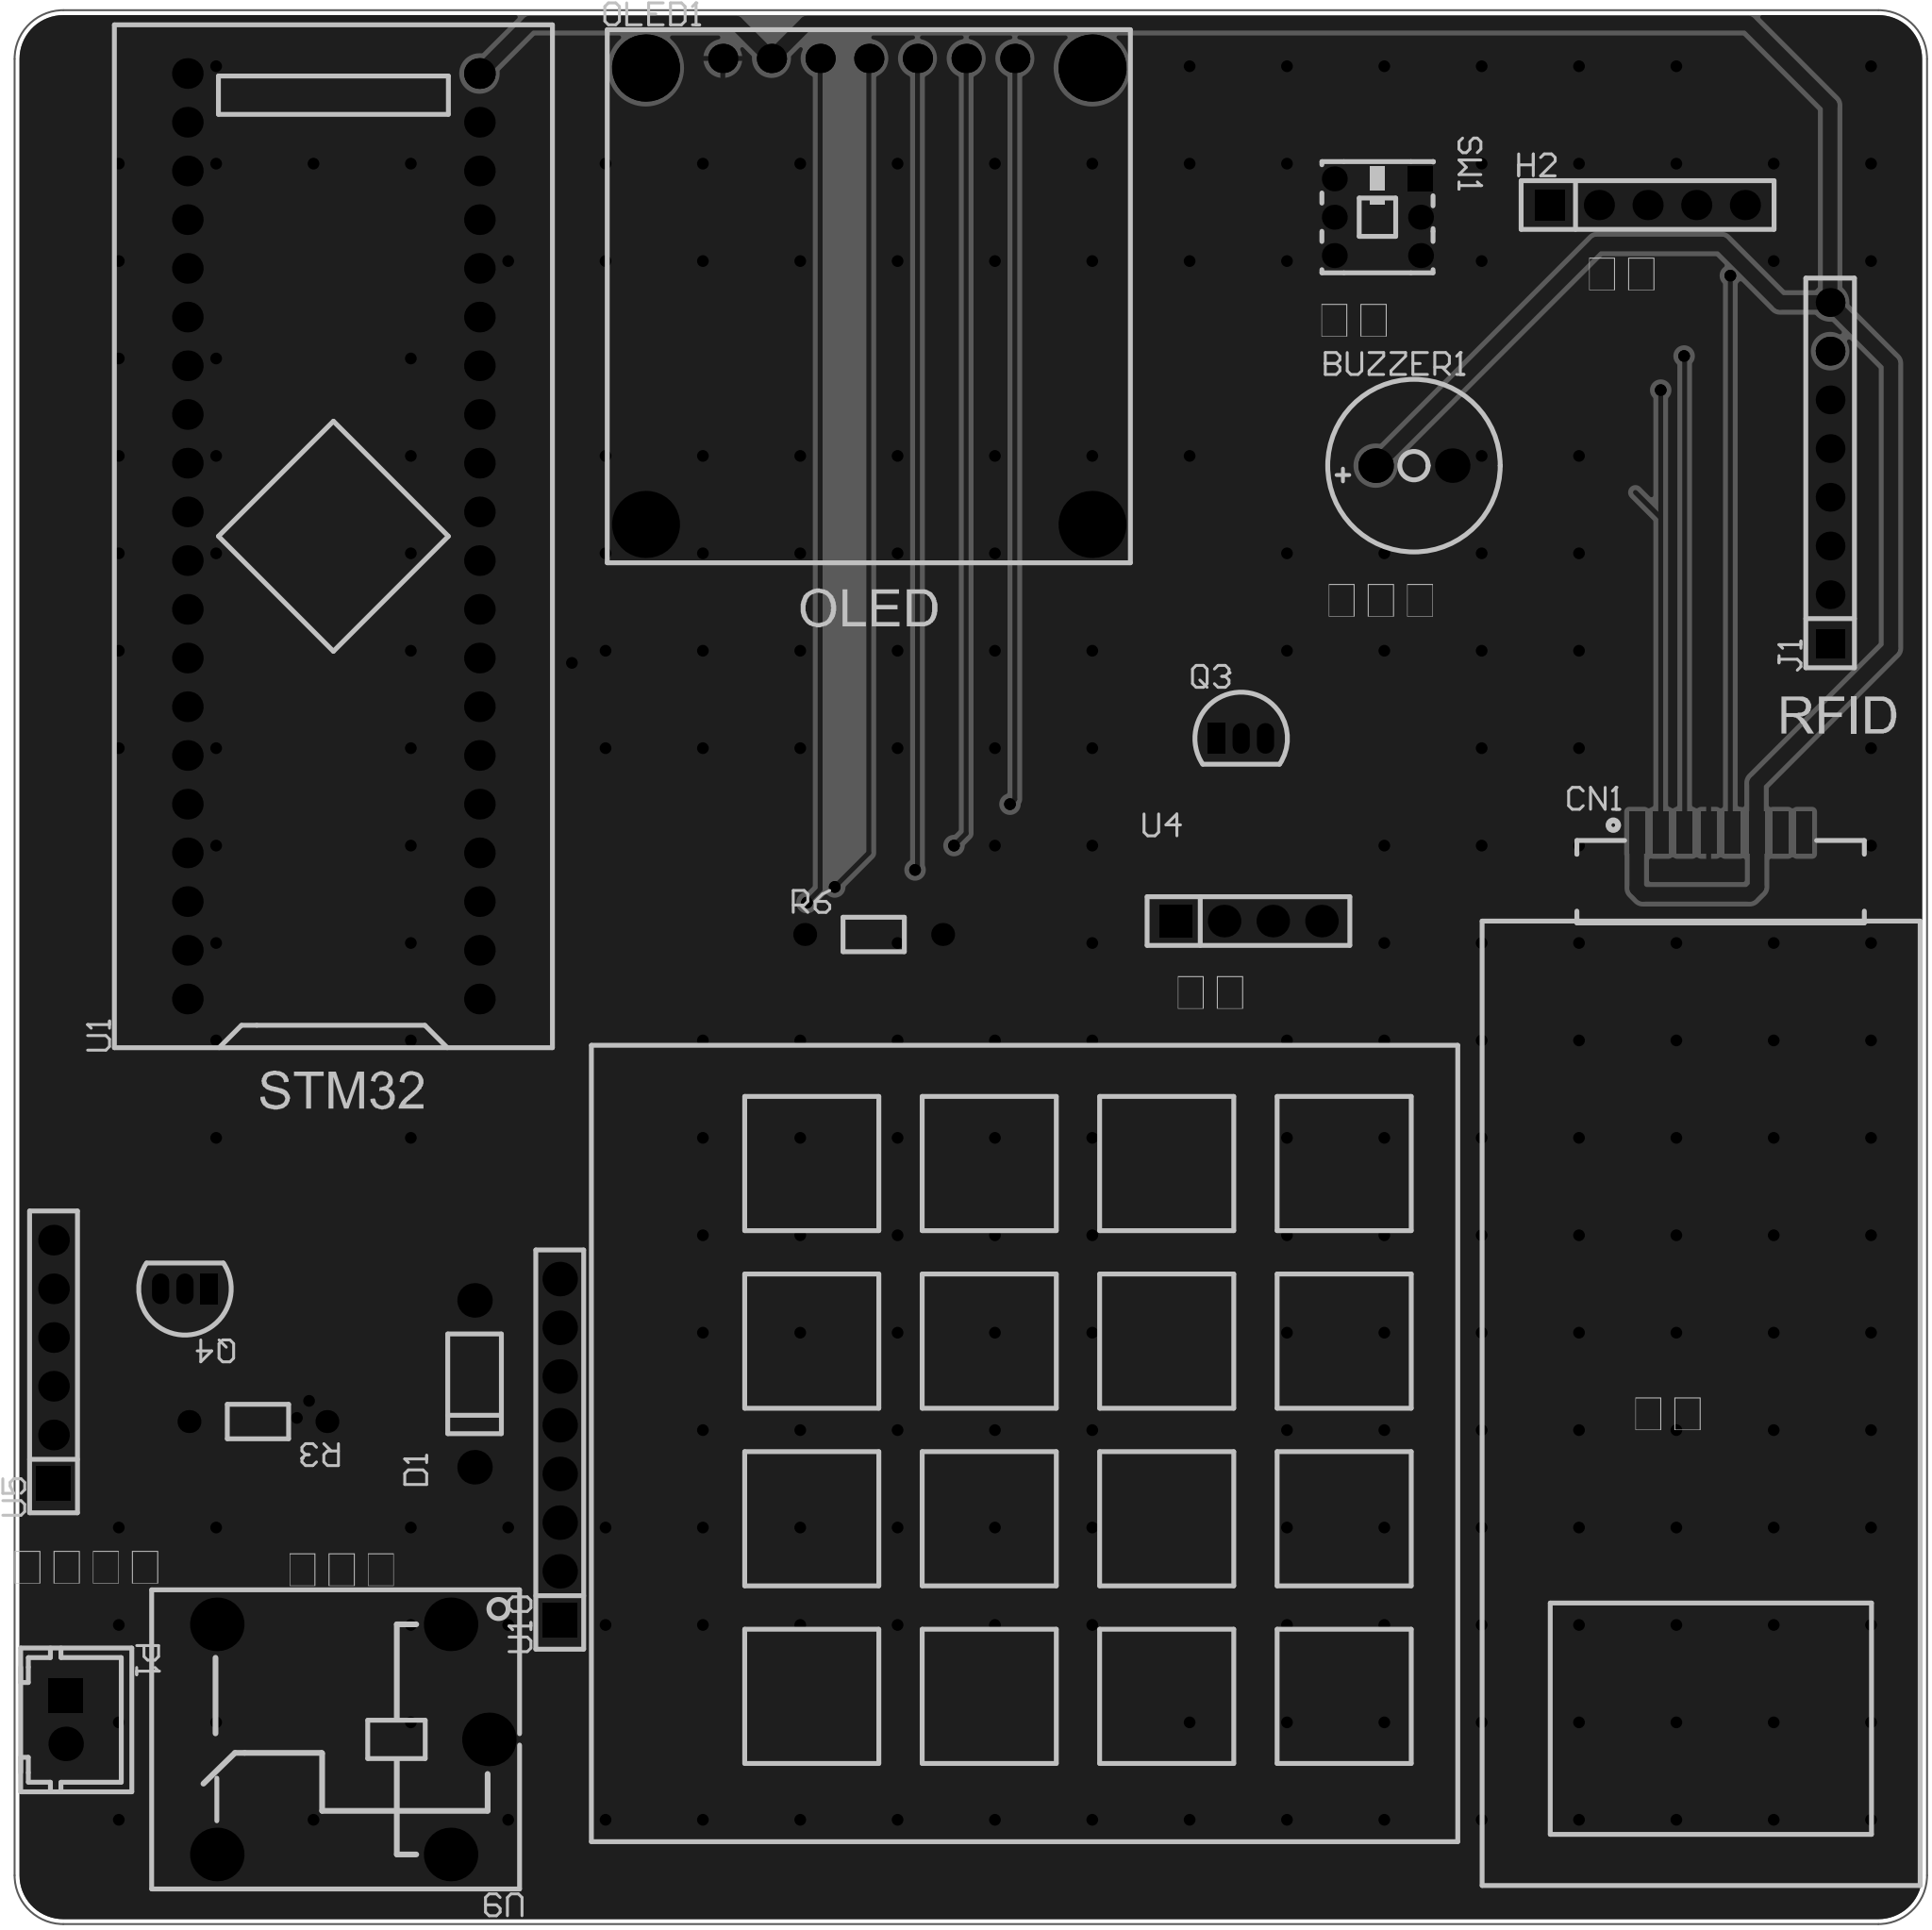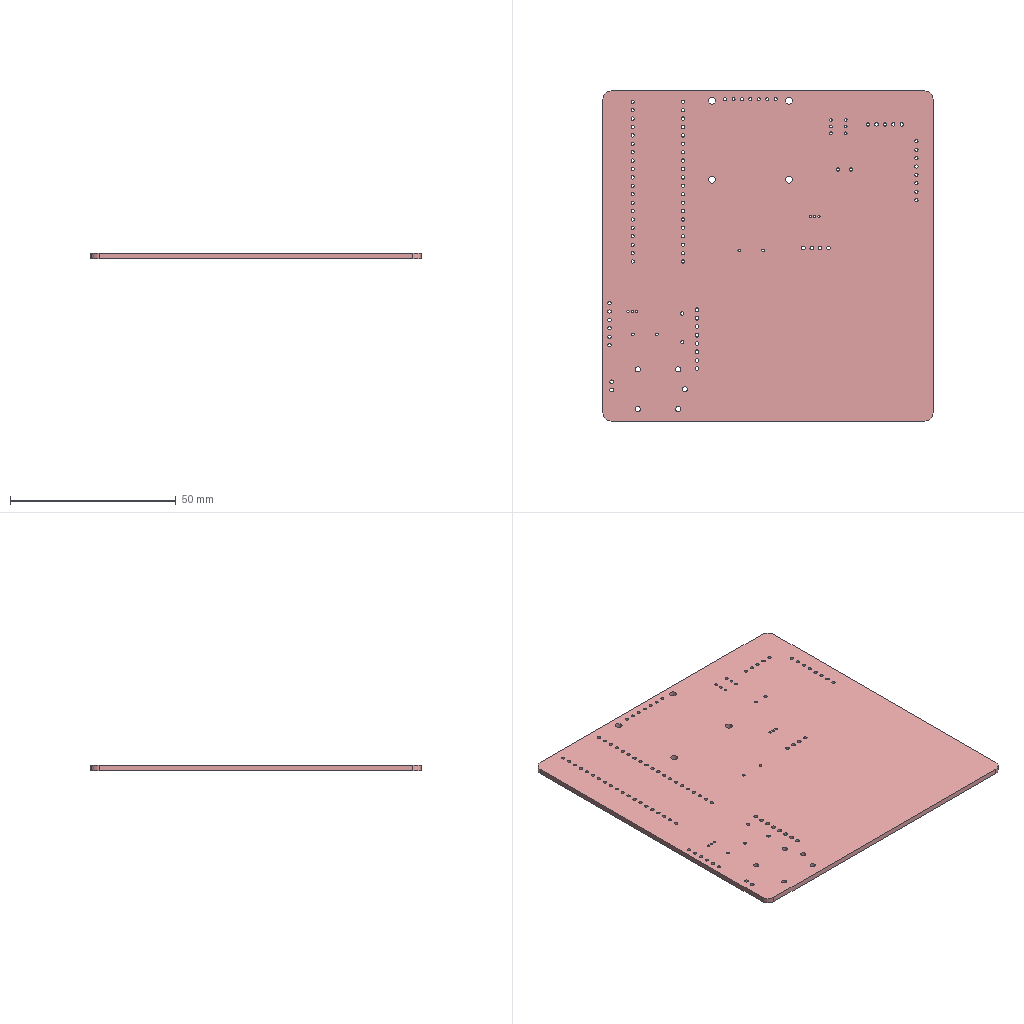Circuit board layout | Altium Designer | box 99.8 x 99.8 x 1.6 mm
Layer stack:
# Altium Designer layer stack of  (unit mm; dielectric type: 0 none, 1 core, 2 prepreg, 3 surface material)
index,name,kind,layer,copper_thickness_mm,dielectric_type,dielectric_thickness_mm,dielectric_material,dielectric_constant
0,Top Paste Mask Layer,other,,,,,,
1,Top Silkscreen Layer,other,,,,,,
2,Top Solder Mask Layer,dielectric,,,3,0.01,,3.3
3,Top Layer,copper,Top Layer,0.035,,,,
4,Dielectric1,dielectric,,,3,1.51,FR4,4.5
5,Bottom Layer,copper,Bottom Layer,0.035,,,,
6,Bottom Solder Mask Layer,dielectric,,,3,0.01,,3.3
7,Bottom Silkscreen Layer,other,,,,,,
8,Bottom Paste Mask Layer,other,,,,,,
# drill layer pairs: low layer,high layer
drill_pair,Top Layer,Bottom Layer
Part placement:
Designator,Comment,Layer,Footprint,Center-X(mm),Center-Y(mm),Rotation
J1,,TopLayer,HDR-TH_8P-P2.54-V-M,175.387,153.924,90
OLED1,,TopLayer,0.96OLED,125.222,163.388,0
U10,,TopLayer,HDR-TH_8P-P2.54-V-F-1,109.093,102.997,90
U1,LCKFB-DKX-STM32F103C8T6,TopLayer,CONN-TH_L53.3-W22.9_STM32F103C8T6-CARD,97.282,150.622,90
U4,,TopLayer,HDR-TH_4P-P2.54-V-F,145.034,130.556,0
Q4,,TopLayer,S8050_TO_92,89.535,111.379,180
R3,1K,TopLayer,Res_1/8W,93.345,104.458,180
D1,,TopLayer,DO_1N4007,104.648,106.426,90
U9,SRD-12VDC-SL-C,TopLayer,RELAY-TH_SRD-XXVDC-XL-C,98.298,87.884,180
R6,1K,TopLayer,Res_1/8W,125.476,129.857,0
BUZZER1,2.7kHz,TopLayer,BUZ-TH_BD9.0-P4.00-D0.6-FD,153.67,154.305,0
Q3,,TopLayer,S8050_TO_92,144.653,140.081,0
H2,,TopLayer,HDR-TH_5P-P2.54-V-F,165.862,167.894,0
P1,WAFER-XH254Z-2A,TopLayer,CONN-TH_2P-P2.50_XH-2A_3045048,83.312,88.9,270
SW1,5.8 WSPT,TopLayer,SW-TH_6P-L5.8-W5.8-P2.00-LS4.5-TL_K8-5851E-L1,151.765,167.259,270
U5,,TopLayer,HDR-TH_6P-P2.54-V-F,82.677,107.569,90
CN1,AS608,TopLayer,AS608,169.672,133.858,0
Pad and via stacks:
# Altium Designer via and pad stacks of  (unit mm). Each distinct definition once, with the count of objects using it.
# via: kind,start_layer,end_layer,hole_mm,diameter_mm,mode(0 simple;1 top-mid-bottom;2 full stack),diameter_per_layer,count,example_net
# pad: kind,layer,hole_mm,hole_type(0 round;1 square;2 slot),plating,top_size,top_shape(1 round;2 rect;3 octagon;9 rounded rect),mid_size,bottom_size,mode,footprint,size_per_layer,count,example
pad,Multi-Layer,1,0,plated,1.5x1.5,2,1.5x1.5,1.5x1.5,0,HDR-TH_8P-P2.54-V-M,,1,J1.1
pad,Multi-Layer,1,0,plated,1.5x1.5,1,1.5x1.5,1.5x1.5,0,HDR-TH_8P-P2.54-V-M,,7,J1.2
pad,Multi-Layer,0.9144,0,plated,1.524x1.524,1,1.524x1.524,1.524x1.524,0,0.96OLED,,7,OLED1.1
pad,Multi-Layer,2.1,0,plated,3.5x3.5,1,3.5x3.5,3.5x3.5,0,0.96OLED,,4,OLED1.0
pad,Multi-Layer,1.2,0,plated,1.8x1.8,2,1.8x1.8,1.8x1.8,0,HDR-TH_8P-P2.54-V-F-1,,1,U10.1
pad,Multi-Layer,1.2,0,plated,1.8x1.8,1,1.8x1.8,1.8x1.8,0,HDR-TH_8P-P2.54-V-F-1,,7,U10.2
pad,Multi-Layer,1,0,plated,1.6x1.6,1,1.6x1.6,1.6x1.6,0,CONN-TH_L53.3-W22.9_STM32F103C8T6-CARD,,40,U1.1
pad,Multi-Layer,1.1,0,plated,1.7x1.7,2,1.7x1.7,1.7x1.7,0,HDR-TH_4P-P2.54-V-F,,1,U4.1
pad,Multi-Layer,1.1,0,plated,1.7x1.7,1,1.7x1.7,1.7x1.7,0,HDR-TH_4P-P2.54-V-F,,3,U4.2
pad,Multi-Layer,0.701,0,plated,0.8992x1.6,2,0.8992x1.6,0.8992x1.6,0,S8050_TO_92,,2,Q4.1
pad,Multi-Layer,0.701,0,plated,0.8992x1.6,1,0.8992x1.6,0.8992x1.6,0,S8050_TO_92,,4,Q4.2
pad,Multi-Layer,0.8001,0,plated,1.199x1.199,1,1.199x1.199,1.199x1.199,0,Res_1/8W,,4,R3.1
pad,Multi-Layer,1,0,plated,1.8x1.8,1,1.8x1.8,1.8x1.8,0,DO_1N4007,,2,D1.1
pad,Multi-Layer,1.524,0,plated,2.794x2.794,1,2.794x2.794,2.794x2.794,0,RELAY-TH_SRD-XXVDC-XL-C,,5,U9.2
pad,Multi-Layer,1,0,plated,1.8x1.8,1,1.8x1.8,1.8x1.8,0,BUZ-TH_BD9.0-P4.00-D0.6-FD,,2,BUZZER1.1
pad,Multi-Layer,1.02,0,plated,1.575x1.575,1,1.575x1.575,1.575x1.575,0,HDR-TH_5P-P2.54-V-F,,4,H2.5
pad,Multi-Layer,1.02,0,plated,1.575x1.575,2,1.575x1.575,1.575x1.575,0,HDR-TH_5P-P2.54-V-F,,1,H2.1
pad,Multi-Layer,1.1,0,plated,1.8x1.8,1,1.8x1.8,1.8x1.8,0,CONN-TH_2P-P2.50_XH-2A_3045048,,1,P1.2
pad,Multi-Layer,1.1,0,plated,1.8x1.8,2,1.8x1.8,1.8x1.8,0,CONN-TH_2P-P2.50_XH-2A_3045048,,1,P1.1
pad,Multi-Layer,0.8,0,plated,1.3x1.3,2,1.3x1.3,1.3x1.3,0,SW-TH_6P-L5.8-W5.8-P2.00-LS4.5-TL_K8-5851E-L1,,1,SW1.1
pad,Multi-Layer,0.8,0,plated,1.3x1.3,1,1.3x1.3,1.3x1.3,0,SW-TH_6P-L5.8-W5.8-P2.00-LS4.5-TL_K8-5851E-L1,,5,SW1.2
pad,Multi-Layer,1.02,0,plated,1.6x1.6,1,1.6x1.6,1.6x1.6,0,HDR-TH_6P-P2.54-V-F,,5,U5.6
pad,Multi-Layer,1.02,0,plated,1.8x1.8,2,1.8x1.8,1.8x1.8,0,HDR-TH_6P-P2.54-V-F,,1,U5.1
pad,Top Layer,0,0,plated,0.8x2.2,2,0.8x2.2,0.8x2.2,0,AS608,,8,CN1.2
pad,Top Layer,0,0,plated,2.35x2.5,2,2.35x2.5,2.35x2.5,0,AS608,,2,CN1.9
via,Top Layer,Bottom Layer,0.3048,0.61,0,,243,OLED_D1
Copper pours:
name,layer,net,type(0 solid;1 hatched;2 none)
Top Layer-GND,Top Layer,GND,0
Bottom Layer-GND,Bottom Layer,GND,0